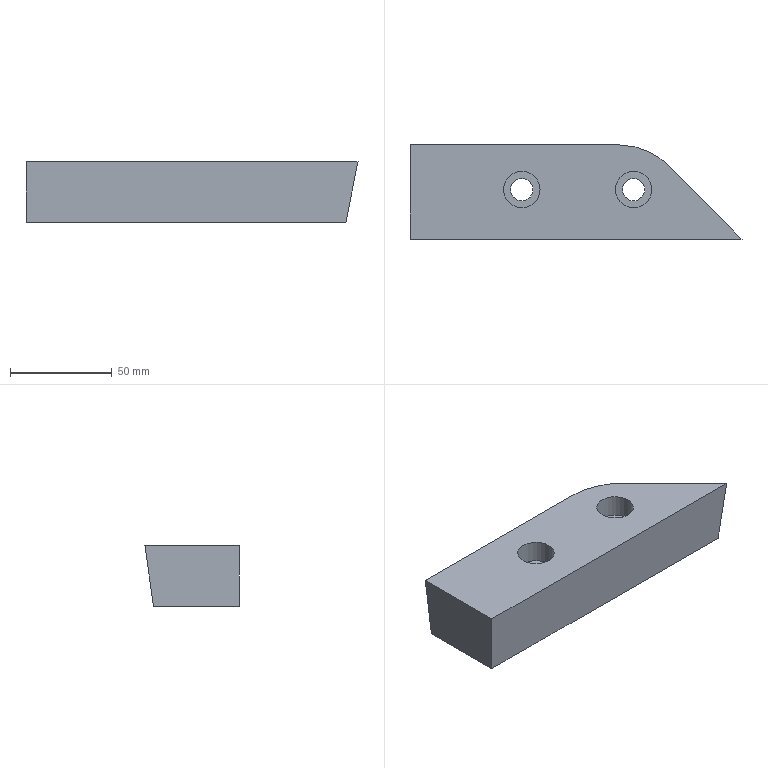Part | STEP file | solid 89 | 1 solid | 13 faces | box 163.329 x 46.356 x 30 mm | volume 173542 mm3 | spline 6 | cylinder 4 | plane 3 | commonest cylinder face diameters 11 x2 18 x2